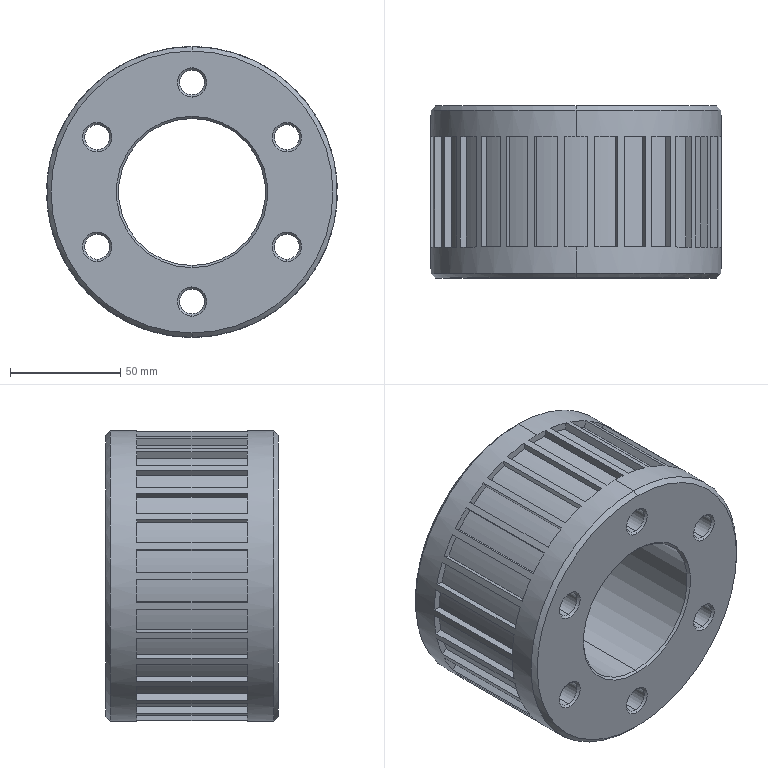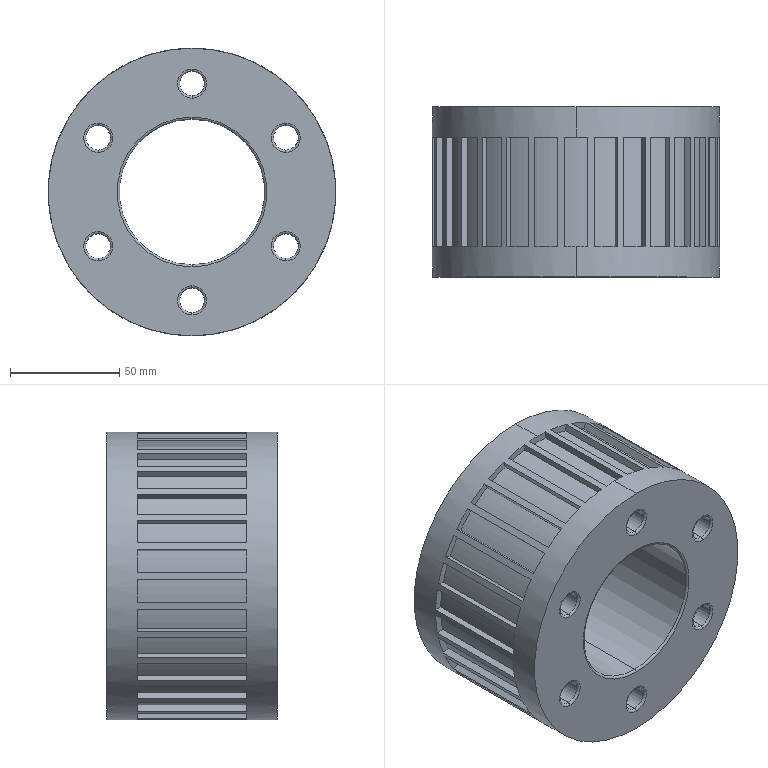Simulation study | ansys workbench
Set-up summary:
category,name,step,type,value,unit,region
solver,ansys_mapdl
solver,version,,,22.1
solver,version,,,22.1
solver,version,,,22.1
solver,version,,,22.1
units,MPA,,stated
analysis,deck1,,transient,transient
load_step,requested,,,1
analysis,nlgeom,,,True
mesh,nodes,,,29762
mesh,elements,,,17336
element_type,ANSYS 187 (type 1),,solid,17010
element_type,ANSYS 154 (type 2),,surface,326
load,load commands in deck,,count,3
bc,support commands in deck,,count,1
named_set,_FIXEDSU,,component
analysis,deck2,,static,static
load_step,requested,,,1
analysis,nlgeom,,,False
mesh,nodes,,,10406
mesh,elements,,,5911
element_type,ANSYS 187 (type 1),,solid,5755
element_type,ANSYS 154 (type 2),,surface,156
load,load commands in deck,,count,3
bc,support commands in deck,,count,1
named_set,_FIXEDSU,,component
named_set,______,,component
analysis,deck3,,transient,transient
load_step,requested,,,1
analysis,nlgeom,,,True
mesh,nodes,,,10406
mesh,elements,,,5911
element_type,ANSYS 187 (type 1),,solid,5755
element_type,ANSYS 154 (type 2),,surface,156
load,load commands in deck,,count,3
bc,support commands in deck,,count,1
named_set,_FIXEDSU,,component
named_set,______,,component
analysis,deck4,,static,static
load_step,requested,,,1
analysis,nlgeom,,,False
mesh,nodes,,,29762
mesh,elements,,,17336
element_type,ANSYS 187 (type 1),,solid,17010
element_type,ANSYS 154 (type 2),,surface,326
load,load commands in deck,,count,3
bc,support commands in deck,,count,1
named_set,_FIXEDSU,,component
material,1,,in results
material,1,,in results
material,1,,in results
material,1,,in results
check,setup vs results,,match,326 surface effect element(s) are not in the reader's mesh and were not compared
check,setup vs results,,match,156 surface effect element(s) are not in the reader's mesh and were not compared
check,setup vs results,,match,156 surface effect element(s) are not in the reader's mesh and were not compared
check,setup vs results,,match,326 surface effect element(s) are not in the reader's mesh and were not compared
Results summary:
result,analysis,,,static
result,last_loadstep,,,1
result,primary field,,,displacement
result,reaction total,1,FX,9e-06,N
result,reaction total,1,FY,500000.014,N
result,reaction total,1,FZ,-5e-06,N
result,mass,,,0.00543,"NMM: mm, ton, N, s, mV, mA, degC"
result,analysis,,,static
result,last_loadstep,,,1
result,primary field,,,displacement
result,reaction total,1,FX,3.2e-05,N
result,reaction total,1,FY,-500000,N
result,reaction total,1,FZ,0.000207,N
result,mass,,,0.005609,"NMM: mm, ton, N, s, mV, mA, degC"
result,analysis,,,static
result,last_loadstep,,,1
result,primary field,,,displacement
result,reaction total,1,FX,-3.6e-05,N
result,reaction total,1,FY,-500000.012,N
result,reaction total,1,FZ,4e-05,N
result,mass,,,0.005609,"NMM: mm, ton, N, s, mV, mA, degC"
result,analysis,,,static
result,last_loadstep,,,1
result,primary field,,,displacement
result,reaction total,1,FX,-0.000145,N
result,reaction total,1,FY,500000,N
result,reaction total,1,FZ,-3e-06,N
result,mass,,,0.00543,"NMM: mm, ton, N, s, mV, mA, degC"